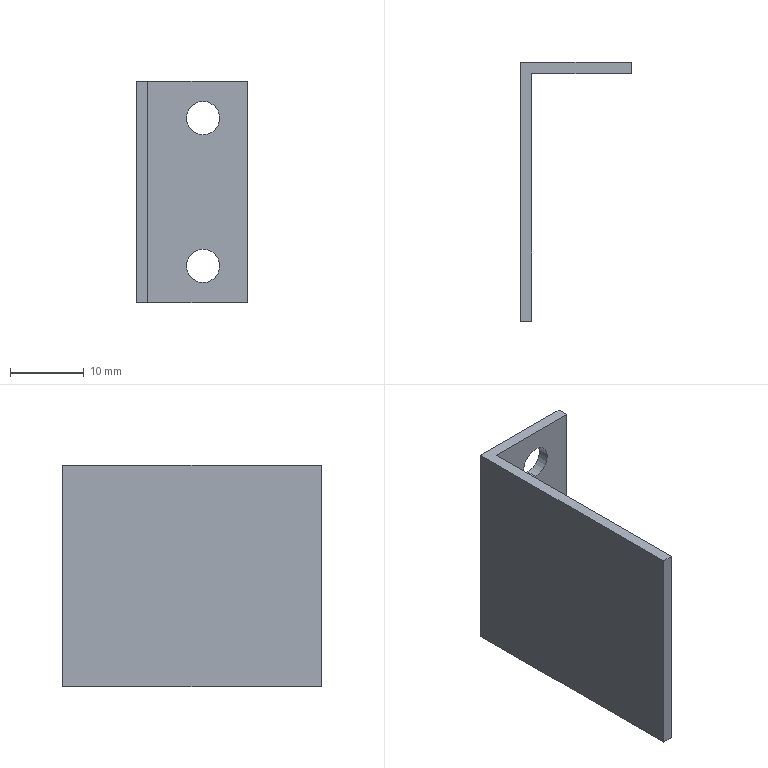Part | STEP file | 0245_210_Dog | 1 solid | 12 faces | box 15 x 35 x 30 mm | volume 2135 mm3 | plane 8 | cylinder 4 | commonest cylinder face diameters 4.5 x4
STEP:
#1=CARTESIAN_POINT('',(0.,0.,0.));
#2=DIRECTION('',(0.,0.,1.));
#3=DIRECTION('',(1.,0.,0.));
#4=AXIS2_PLACEMENT_3D('',#1,#2,#3);
#5=CARTESIAN_POINT('',(9.,-1.5,12.25));
#6=VERTEX_POINT('',#5);
#7=CARTESIAN_POINT('',(9.,0.,12.25));
#8=VERTEX_POINT('',#7);
#9=CARTESIAN_POINT('',(9.,0.,12.25));
#10=DIRECTION('',(0.,1.,0.));
#11=VECTOR('',#10,1.);
#12=LINE('',#9,#11);
#13=CARTESIAN_POINT('',(9.,0.,10.));
#14=DIRECTION('',(0.,1.,0.));
#15=DIRECTION('',(0.,0.,1.));
#16=AXIS2_PLACEMENT_3D('',#13,#14,#15);
#17=CYLINDRICAL_SURFACE('',#16,2.25);
#18=CARTESIAN_POINT('',(6.283,0.));
#19=DIRECTION('',(0.,1.));
#20=VECTOR('',#19,1.);
#21=LINE('',#18,#20);
#22=(GEOMETRIC_REPRESENTATION_CONTEXT(2)PARAMETRIC_REPRESENTATION_CONTEXT()REPRESENTATION_CONTEXT('',''));
#23=DEFINITIONAL_REPRESENTATION('',(#21),#22);
#24=PCURVE('',#17,#23);
#25=CARTESIAN_POINT('',(9.,0.,10.));
#26=DIRECTION('',(0.,1.,0.));
#27=DIRECTION('',(0.,0.,1.));
#28=AXIS2_PLACEMENT_3D('',#25,#26,#27);
#29=CYLINDRICAL_SURFACE('',#28,2.25);
#30=CARTESIAN_POINT('',(0.,0.));
#31=DIRECTION('',(0.,1.));
#32=VECTOR('',#31,1.);
#33=LINE('',#30,#32);
#34=(GEOMETRIC_REPRESENTATION_CONTEXT(2)PARAMETRIC_REPRESENTATION_CONTEXT()REPRESENTATION_CONTEXT('',''));
#35=DEFINITIONAL_REPRESENTATION('',(#33),#34);
#36=PCURVE('',#29,#35);
#37=SURFACE_CURVE('',#12,(#24,#36),.PCURVE_S1.);
#38=EDGE_CURVE('',#6,#8,#37,.T.);
#39=ORIENTED_EDGE('',*,*,#38,.T.);
#40=CARTESIAN_POINT('',(9.,0.,7.75));
#41=VERTEX_POINT('',#40);
#42=CARTESIAN_POINT('',(9.,0.,10.));
#43=DIRECTION('',(0.,1.,0.));
#44=DIRECTION('',(0.,0.,1.));
#45=AXIS2_PLACEMENT_3D('',#42,#43,#44);
#46=CIRCLE('',#45,2.25);
#47=CARTESIAN_POINT('',(0.,0.));
#48=DIRECTION('',(1.,0.));
#49=VECTOR('',#48,1.);
#50=LINE('',#47,#49);
#51=(GEOMETRIC_REPRESENTATION_CONTEXT(2)PARAMETRIC_REPRESENTATION_CONTEXT()REPRESENTATION_CONTEXT('',''));
#52=DEFINITIONAL_REPRESENTATION('',(#50),#51);
#53=PCURVE('',#17,#52);
#54=CARTESIAN_POINT('',(15.,0.,15.));
#55=DIRECTION('',(0.,-1.,0.));
#56=DIRECTION('',(1.,0.,0.));
#57=AXIS2_PLACEMENT_3D('',#54,#55,#56);
#58=PLANE('',#57);
#59=CARTESIAN_POINT('',(-6.,-2.75));
#60=CARTESIAN_POINT('',(-2.103,-2.75));
#61=CARTESIAN_POINT('',(-4.051,-6.125));
#62=CARTESIAN_POINT('',(-6.,-9.5));
#63=CARTESIAN_POINT('',(-7.949,-6.125));
#64=CARTESIAN_POINT('',(-9.897,-2.75));
#65=CARTESIAN_POINT('',(-6.,-2.75));
#66=(BOUNDED_CURVE()B_SPLINE_CURVE(2,(#59,#60,#61,#62,#63,#64,#65),.UNSPECIFIED.,.T.,.F.)B_SPLINE_CURVE_WITH_KNOTS((1,2,2,2,2,1),(-2.094,0.,2.094,4.189,6.283,8.378),.UNSPECIFIED.)CURVE()GEOMETRIC_REPRESENTATION_ITEM()RATIONAL_B_SPLINE_CURVE((1.,0.5,1.,0.5,1.,0.5,1.))REPRESENTATION_ITEM(''));
#67=(GEOMETRIC_REPRESENTATION_CONTEXT(2)PARAMETRIC_REPRESENTATION_CONTEXT()REPRESENTATION_CONTEXT('',''));
#68=DEFINITIONAL_REPRESENTATION('',(#66),#67);
#69=PCURVE('',#58,#68);
#70=SURFACE_CURVE('',#46,(#53,#69),.PCURVE_S1.);
#71=EDGE_CURVE('',#41,#8,#70,.T.);
#72=ORIENTED_EDGE('',*,*,#71,.F.);
#73=CARTESIAN_POINT('',(9.,-1.5,7.75));
#74=VERTEX_POINT('',#73);
#75=CARTESIAN_POINT('',(9.,0.,7.75));
#76=DIRECTION('',(0.,1.,0.));
#77=VECTOR('',#76,1.);
#78=LINE('',#75,#77);
#79=CARTESIAN_POINT('',(3.142,0.));
#80=DIRECTION('',(0.,1.));
#81=VECTOR('',#80,1.);
#82=LINE('',#79,#81);
#83=(GEOMETRIC_REPRESENTATION_CONTEXT(2)PARAMETRIC_REPRESENTATION_CONTEXT()REPRESENTATION_CONTEXT('',''));
#84=DEFINITIONAL_REPRESENTATION('',(#82),#83);
#85=PCURVE('',#17,#84);
#86=CARTESIAN_POINT('',(3.142,0.));
#87=DIRECTION('',(0.,1.));
#88=VECTOR('',#87,1.);
#89=LINE('',#86,#88);
#90=(GEOMETRIC_REPRESENTATION_CONTEXT(2)PARAMETRIC_REPRESENTATION_CONTEXT()REPRESENTATION_CONTEXT('',''));
#91=DEFINITIONAL_REPRESENTATION('',(#89),#90);
#92=PCURVE('',#29,#91);
#93=SURFACE_CURVE('',#78,(#85,#92),.PCURVE_S1.);
#94=EDGE_CURVE('',#74,#41,#93,.T.);
#95=ORIENTED_EDGE('',*,*,#94,.F.);
#96=CARTESIAN_POINT('',(9.,-1.5,10.));
#97=DIRECTION('',(0.,1.,0.));
#98=DIRECTION('',(-1.,0.,0.));
#99=AXIS2_PLACEMENT_3D('',#96,#97,#98);
#100=CIRCLE('',#99,2.25);
#101=CARTESIAN_POINT('',(-1.571,-1.5));
#102=DIRECTION('',(1.,0.));
#103=VECTOR('',#102,1.);
#104=LINE('',#101,#103);
#105=(GEOMETRIC_REPRESENTATION_CONTEXT(2)PARAMETRIC_REPRESENTATION_CONTEXT()REPRESENTATION_CONTEXT('',''));
#106=DEFINITIONAL_REPRESENTATION('',(#104),#105);
#107=PCURVE('',#17,#106);
#108=CARTESIAN_POINT('',(1.5,-1.5,15.));
#109=DIRECTION('',(0.,1.,0.));
#110=DIRECTION('',(-1.,0.,0.));
#111=AXIS2_PLACEMENT_3D('',#108,#109,#110);
#112=PLANE('',#111);
#113=CARTESIAN_POINT('',(-7.5,-5.));
#114=DIRECTION('',(1.,0.));
#115=AXIS2_PLACEMENT_2D('',#113,#114);
#116=CIRCLE('',#115,2.25);
#117=(GEOMETRIC_REPRESENTATION_CONTEXT(2)PARAMETRIC_REPRESENTATION_CONTEXT()REPRESENTATION_CONTEXT('',''));
#118=DEFINITIONAL_REPRESENTATION('',(#116),#117);
#119=PCURVE('',#112,#118);
#120=SURFACE_CURVE('',#100,(#107,#119),.PCURVE_S1.);
#121=EDGE_CURVE('',#74,#6,#120,.T.);
#122=ORIENTED_EDGE('',*,*,#121,.T.);
#123=EDGE_LOOP('',(#39,#72,#95,#122));
#124=FACE_BOUND('',#123,.F.);
#125=ADVANCED_FACE('',(#124),#17,.F.);
#126=CARTESIAN_POINT('',(9.,-1.5,-7.75));
#127=VERTEX_POINT('',#126);
#128=CARTESIAN_POINT('',(9.,0.,-7.75));
#129=VERTEX_POINT('',#128);
#130=CARTESIAN_POINT('',(9.,0.,-7.75));
#131=DIRECTION('',(0.,1.,0.));
#132=VECTOR('',#131,1.);
#133=LINE('',#130,#132);
#134=CARTESIAN_POINT('',(9.,0.,-10.));
#135=DIRECTION('',(0.,1.,0.));
#136=DIRECTION('',(0.,0.,1.));
#137=AXIS2_PLACEMENT_3D('',#134,#135,#136);
#138=CYLINDRICAL_SURFACE('',#137,2.25);
#139=CARTESIAN_POINT('',(6.283,0.));
#140=DIRECTION('',(0.,1.));
#141=VECTOR('',#140,1.);
#142=LINE('',#139,#141);
#143=(GEOMETRIC_REPRESENTATION_CONTEXT(2)PARAMETRIC_REPRESENTATION_CONTEXT()REPRESENTATION_CONTEXT('',''));
#144=DEFINITIONAL_REPRESENTATION('',(#142),#143);
#145=PCURVE('',#138,#144);
#146=CARTESIAN_POINT('',(9.,0.,-10.));
#147=DIRECTION('',(0.,1.,0.));
#148=DIRECTION('',(0.,0.,1.));
#149=AXIS2_PLACEMENT_3D('',#146,#147,#148);
#150=CYLINDRICAL_SURFACE('',#149,2.25);
#151=CARTESIAN_POINT('',(0.,0.));
#152=DIRECTION('',(0.,1.));
#153=VECTOR('',#152,1.);
#154=LINE('',#151,#153);
#155=(GEOMETRIC_REPRESENTATION_CONTEXT(2)PARAMETRIC_REPRESENTATION_CONTEXT()REPRESENTATION_CONTEXT('',''));
#156=DEFINITIONAL_REPRESENTATION('',(#154),#155);
#157=PCURVE('',#150,#156);
#158=SURFACE_CURVE('',#133,(#145,#157),.PCURVE_S1.);
#159=EDGE_CURVE('',#127,#129,#158,.T.);
#160=ORIENTED_EDGE('',*,*,#159,.T.);
#161=CARTESIAN_POINT('',(9.,0.,-12.25));
#162=VERTEX_POINT('',#161);
#163=CARTESIAN_POINT('',(9.,0.,-10.));
#164=DIRECTION('',(0.,1.,0.));
#165=DIRECTION('',(0.,0.,1.));
#166=AXIS2_PLACEMENT_3D('',#163,#164,#165);
#167=CIRCLE('',#166,2.25);
#168=CARTESIAN_POINT('',(0.,0.));
#169=DIRECTION('',(1.,0.));
#170=VECTOR('',#169,1.);
#171=LINE('',#168,#170);
#172=(GEOMETRIC_REPRESENTATION_CONTEXT(2)PARAMETRIC_REPRESENTATION_CONTEXT()REPRESENTATION_CONTEXT('',''));
#173=DEFINITIONAL_REPRESENTATION('',(#171),#172);
#174=PCURVE('',#138,#173);
#175=CARTESIAN_POINT('',(-6.,-22.75));
#176=CARTESIAN_POINT('',(-2.103,-22.75));
#177=CARTESIAN_POINT('',(-4.051,-26.125));
#178=CARTESIAN_POINT('',(-6.,-29.5));
#179=CARTESIAN_POINT('',(-7.949,-26.125));
#180=CARTESIAN_POINT('',(-9.897,-22.75));
#181=CARTESIAN_POINT('',(-6.,-22.75));
#182=(BOUNDED_CURVE()B_SPLINE_CURVE(2,(#175,#176,#177,#178,#179,#180,#181),.UNSPECIFIED.,.T.,.F.)B_SPLINE_CURVE_WITH_KNOTS((1,2,2,2,2,1),(-2.094,0.,2.094,4.189,6.283,8.378),.UNSPECIFIED.)CURVE()GEOMETRIC_REPRESENTATION_ITEM()RATIONAL_B_SPLINE_CURVE((1.,0.5,1.,0.5,1.,0.5,1.))REPRESENTATION_ITEM(''));
#183=(GEOMETRIC_REPRESENTATION_CONTEXT(2)PARAMETRIC_REPRESENTATION_CONTEXT()REPRESENTATION_CONTEXT('',''));
#184=DEFINITIONAL_REPRESENTATION('',(#182),#183);
#185=PCURVE('',#58,#184);
#186=SURFACE_CURVE('',#167,(#174,#185),.PCURVE_S1.);
#187=EDGE_CURVE('',#162,#129,#186,.T.);
#188=ORIENTED_EDGE('',*,*,#187,.F.);
#189=CARTESIAN_POINT('',(9.,-1.5,-12.25));
#190=VERTEX_POINT('',#189);
#191=CARTESIAN_POINT('',(9.,0.,-12.25));
#192=DIRECTION('',(0.,1.,0.));
#193=VECTOR('',#192,1.);
#194=LINE('',#191,#193);
#195=CARTESIAN_POINT('',(3.142,0.));
#196=DIRECTION('',(0.,1.));
#197=VECTOR('',#196,1.);
#198=LINE('',#195,#197);
#199=(GEOMETRIC_REPRESENTATION_CONTEXT(2)PARAMETRIC_REPRESENTATION_CONTEXT()REPRESENTATION_CONTEXT('',''));
#200=DEFINITIONAL_REPRESENTATION('',(#198),#199);
#201=PCURVE('',#138,#200);
#202=CARTESIAN_POINT('',(3.142,0.));
#203=DIRECTION('',(0.,1.));
#204=VECTOR('',#203,1.);
#205=LINE('',#202,#204);
#206=(GEOMETRIC_REPRESENTATION_CONTEXT(2)PARAMETRIC_REPRESENTATION_CONTEXT()REPRESENTATION_CONTEXT('',''));
#207=DEFINITIONAL_REPRESENTATION('',(#205),#206);
#208=PCURVE('',#150,#207);
#209=SURFACE_CURVE('',#194,(#201,#208),.PCURVE_S1.);
#210=EDGE_CURVE('',#190,#162,#209,.T.);
#211=ORIENTED_EDGE('',*,*,#210,.F.);
#212=CARTESIAN_POINT('',(9.,-1.5,-10.));
#213=DIRECTION('',(0.,1.,0.));
#214=DIRECTION('',(-1.,0.,0.));
#215=AXIS2_PLACEMENT_3D('',#212,#213,#214);
#216=CIRCLE('',#215,2.25);
#217=CARTESIAN_POINT('',(-1.571,-1.5));
#218=DIRECTION('',(1.,0.));
#219=VECTOR('',#218,1.);
#220=LINE('',#217,#219);
#221=(GEOMETRIC_REPRESENTATION_CONTEXT(2)PARAMETRIC_REPRESENTATION_CONTEXT()REPRESENTATION_CONTEXT('',''));
#222=DEFINITIONAL_REPRESENTATION('',(#220),#221);
#223=PCURVE('',#138,#222);
#224=CARTESIAN_POINT('',(-7.5,-25.));
#225=DIRECTION('',(1.,0.));
#226=AXIS2_PLACEMENT_2D('',#224,#225);
#227=CIRCLE('',#226,2.25);
#228=(GEOMETRIC_REPRESENTATION_CONTEXT(2)PARAMETRIC_REPRESENTATION_CONTEXT()REPRESENTATION_CONTEXT('',''));
#229=DEFINITIONAL_REPRESENTATION('',(#227),#228);
#230=PCURVE('',#112,#229);
#231=SURFACE_CURVE('',#216,(#223,#230),.PCURVE_S1.);
#232=EDGE_CURVE('',#190,#127,#231,.T.);
#233=ORIENTED_EDGE('',*,*,#232,.T.);
#234=EDGE_LOOP('',(#160,#188,#211,#233));
#235=FACE_BOUND('',#234,.F.);
#236=ADVANCED_FACE('',(#235),#138,.F.);
#237=CARTESIAN_POINT('',(9.,0.,10.));
#238=DIRECTION('',(0.,1.,0.));
#239=DIRECTION('',(0.,0.,1.));
#240=AXIS2_PLACEMENT_3D('',#237,#238,#239);
#241=CIRCLE('',#240,2.25);
#242=CARTESIAN_POINT('',(-6.,-2.75));
#243=CARTESIAN_POINT('',(-2.103,-2.75));
#244=CARTESIAN_POINT('',(-4.051,-6.125));
#245=CARTESIAN_POINT('',(-6.,-9.5));
#246=CARTESIAN_POINT('',(-7.949,-6.125));
#247=CARTESIAN_POINT('',(-9.897,-2.75));
#248=CARTESIAN_POINT('',(-6.,-2.75));
#249=(BOUNDED_CURVE()B_SPLINE_CURVE(2,(#242,#243,#244,#245,#246,#247,#248),.UNSPECIFIED.,.T.,.F.)B_SPLINE_CURVE_WITH_KNOTS((1,2,2,2,2,1),(-2.094,0.,2.094,4.189,6.283,8.378),.UNSPECIFIED.)CURVE()GEOMETRIC_REPRESENTATION_ITEM()RATIONAL_B_SPLINE_CURVE((1.,0.5,1.,0.5,1.,0.5,1.))REPRESENTATION_ITEM(''));
#250=(GEOMETRIC_REPRESENTATION_CONTEXT(2)PARAMETRIC_REPRESENTATION_CONTEXT()REPRESENTATION_CONTEXT('',''));
#251=DEFINITIONAL_REPRESENTATION('',(#249),#250);
#252=PCURVE('',#58,#251);
#253=CARTESIAN_POINT('',(0.,0.));
#254=DIRECTION('',(1.,0.));
#255=VECTOR('',#254,1.);
#256=LINE('',#253,#255);
#257=(GEOMETRIC_REPRESENTATION_CONTEXT(2)PARAMETRIC_REPRESENTATION_CONTEXT()REPRESENTATION_CONTEXT('',''));
#258=DEFINITIONAL_REPRESENTATION('',(#256),#257);
#259=PCURVE('',#29,#258);
#260=SURFACE_CURVE('',#241,(#252,#259),.PCURVE_S1.);
#261=EDGE_CURVE('',#8,#41,#260,.T.);
#262=ORIENTED_EDGE('',*,*,#261,.F.);
#263=ORIENTED_EDGE('',*,*,#71,.F.);
#264=EDGE_LOOP('',(#262,#263));
#265=FACE_BOUND('',#264,.T.);
#266=CARTESIAN_POINT('',(9.,0.,-10.));
#267=DIRECTION('',(0.,1.,0.));
#268=DIRECTION('',(0.,0.,1.));
#269=AXIS2_PLACEMENT_3D('',#266,#267,#268);
#270=CIRCLE('',#269,2.25);
#271=CARTESIAN_POINT('',(-6.,-22.75));
#272=CARTESIAN_POINT('',(-2.103,-22.75));
#273=CARTESIAN_POINT('',(-4.051,-26.125));
#274=CARTESIAN_POINT('',(-6.,-29.5));
#275=CARTESIAN_POINT('',(-7.949,-26.125));
#276=CARTESIAN_POINT('',(-9.897,-22.75));
#277=CARTESIAN_POINT('',(-6.,-22.75));
#278=(BOUNDED_CURVE()B_SPLINE_CURVE(2,(#271,#272,#273,#274,#275,#276,#277),.UNSPECIFIED.,.T.,.F.)B_SPLINE_CURVE_WITH_KNOTS((1,2,2,2,2,1),(-2.094,0.,2.094,4.189,6.283,8.378),.UNSPECIFIED.)CURVE()GEOMETRIC_REPRESENTATION_ITEM()RATIONAL_B_SPLINE_CURVE((1.,0.5,1.,0.5,1.,0.5,1.))REPRESENTATION_ITEM(''));
#279=(GEOMETRIC_REPRESENTATION_CONTEXT(2)PARAMETRIC_REPRESENTATION_CONTEXT()REPRESENTATION_CONTEXT('',''));
#280=DEFINITIONAL_REPRESENTATION('',(#278),#279);
#281=PCURVE('',#58,#280);
#282=CARTESIAN_POINT('',(0.,0.));
#283=DIRECTION('',(1.,0.));
#284=VECTOR('',#283,1.);
#285=LINE('',#282,#284);
#286=(GEOMETRIC_REPRESENTATION_CONTEXT(2)PARAMETRIC_REPRESENTATION_CONTEXT()REPRESENTATION_CONTEXT('',''));
#287=DEFINITIONAL_REPRESENTATION('',(#285),#286);
#288=PCURVE('',#150,#287);
#289=SURFACE_CURVE('',#270,(#281,#288),.PCURVE_S1.);
#290=EDGE_CURVE('',#129,#162,#289,.T.);
#291=ORIENTED_EDGE('',*,*,#290,.F.);
#292=ORIENTED_EDGE('',*,*,#187,.F.);
#293=EDGE_LOOP('',(#291,#292));
#294=FACE_BOUND('',#293,.T.);
#295=CARTESIAN_POINT('',(15.,0.,-15.));
#296=VERTEX_POINT('',#295);
#297=CARTESIAN_POINT('',(0.,0.,-15.));
#298=VERTEX_POINT('',#297);
#299=CARTESIAN_POINT('',(15.,0.,-15.));
#300=DIRECTION('',(-1.,0.,0.));
#301=VECTOR('',#300,1.);
#302=LINE('',#299,#301);
#303=CARTESIAN_POINT('',(0.,-30.));
#304=DIRECTION('',(-1.,0.));
#305=VECTOR('',#304,1.);
#306=LINE('',#303,#305);
#307=(GEOMETRIC_REPRESENTATION_CONTEXT(2)PARAMETRIC_REPRESENTATION_CONTEXT()REPRESENTATION_CONTEXT('',''));
#308=DEFINITIONAL_REPRESENTATION('',(#306),#307);
#309=PCURVE('',#58,#308);
#310=CARTESIAN_POINT('',(0.,0.,-15.));
#311=DIRECTION('',(0.,0.,1.));
#312=DIRECTION('',(1.,0.,0.));
#313=AXIS2_PLACEMENT_3D('',#310,#311,#312);
#314=PLANE('',#313);
#315=CARTESIAN_POINT('',(15.,0.));
#316=DIRECTION('',(-1.,0.));
#317=VECTOR('',#316,1.);
#318=LINE('',#315,#317);
#319=(GEOMETRIC_REPRESENTATION_CONTEXT(2)PARAMETRIC_REPRESENTATION_CONTEXT()REPRESENTATION_CONTEXT('',''));
#320=DEFINITIONAL_REPRESENTATION('',(#318),#319);
#321=PCURVE('',#314,#320);
#322=SURFACE_CURVE('',#302,(#309,#321),.PCURVE_S1.);
#323=EDGE_CURVE('',#296,#298,#322,.T.);
#324=ORIENTED_EDGE('',*,*,#323,.T.);
#325=CARTESIAN_POINT('',(0.,0.,15.));
#326=VERTEX_POINT('',#325);
#327=CARTESIAN_POINT('',(0.,0.,15.));
#328=DIRECTION('',(0.,0.,-1.));
#329=VECTOR('',#328,1.);
#330=LINE('',#327,#329);
#331=CARTESIAN_POINT('',(-15.,0.));
#332=DIRECTION('',(0.,-1.));
#333=VECTOR('',#332,1.);
#334=LINE('',#331,#333);
#335=(GEOMETRIC_REPRESENTATION_CONTEXT(2)PARAMETRIC_REPRESENTATION_CONTEXT()REPRESENTATION_CONTEXT('',''));
#336=DEFINITIONAL_REPRESENTATION('',(#334),#335);
#337=PCURVE('',#58,#336);
#338=CARTESIAN_POINT('',(0.,0.,15.));
#339=DIRECTION('',(1.,0.,0.));
#340=DIRECTION('',(0.,1.,0.));
#341=AXIS2_PLACEMENT_3D('',#338,#339,#340);
#342=PLANE('',#341);
#343=CARTESIAN_POINT('',(0.,0.));
#344=DIRECTION('',(0.,-1.));
#345=VECTOR('',#344,1.);
#346=LINE('',#343,#345);
#347=(GEOMETRIC_REPRESENTATION_CONTEXT(2)PARAMETRIC_REPRESENTATION_CONTEXT()REPRESENTATION_CONTEXT('',''));
#348=DEFINITIONAL_REPRESENTATION('',(#346),#347);
#349=PCURVE('',#342,#348);
#350=SURFACE_CURVE('',#330,(#337,#349),.PCURVE_S1.);
#351=EDGE_CURVE('',#326,#298,#350,.T.);
#352=ORIENTED_EDGE('',*,*,#351,.F.);
#353=CARTESIAN_POINT('',(15.,0.,15.));
#354=VERTEX_POINT('',#353);
#355=CARTESIAN_POINT('',(15.,0.,15.));
#356=DIRECTION('',(-1.,0.,0.));
#357=VECTOR('',#356,1.);
#358=LINE('',#355,#357);
#359=CARTESIAN_POINT('',(0.,0.));
#360=DIRECTION('',(-1.,0.));
#361=VECTOR('',#360,1.);
#362=LINE('',#359,#361);
#363=(GEOMETRIC_REPRESENTATION_CONTEXT(2)PARAMETRIC_REPRESENTATION_CONTEXT()REPRESENTATION_CONTEXT('',''));
#364=DEFINITIONAL_REPRESENTATION('',(#362),#363);
#365=PCURVE('',#58,#364);
#366=CARTESIAN_POINT('',(0.,0.,15.));
#367=DIRECTION('',(0.,0.,1.));
#368=DIRECTION('',(1.,0.,0.));
#369=AXIS2_PLACEMENT_3D('',#366,#367,#368);
#370=PLANE('',#369);
#371=CARTESIAN_POINT('',(15.,0.));
#372=DIRECTION('',(-1.,0.));
#373=VECTOR('',#372,1.);
#374=LINE('',#371,#373);
#375=(GEOMETRIC_REPRESENTATION_CONTEXT(2)PARAMETRIC_REPRESENTATION_CONTEXT()REPRESENTATION_CONTEXT('',''));
#376=DEFINITIONAL_REPRESENTATION('',(#374),#375);
#377=PCURVE('',#370,#376);
#378=SURFACE_CURVE('',#358,(#365,#377),.PCURVE_S1.);
#379=EDGE_CURVE('',#354,#326,#378,.T.);
#380=ORIENTED_EDGE('',*,*,#379,.F.);
#381=CARTESIAN_POINT('',(15.,0.,15.));
#382=DIRECTION('',(0.,0.,-1.));
#383=VECTOR('',#382,1.);
#384=LINE('',#381,#383);
#385=CARTESIAN_POINT('',(0.,0.));
#386=DIRECTION('',(0.,-1.));
#387=VECTOR('',#386,1.);
#388=LINE('',#385,#387);
#389=(GEOMETRIC_REPRESENTATION_CONTEXT(2)PARAMETRIC_REPRESENTATION_CONTEXT()REPRESENTATION_CONTEXT('',''));
#390=DEFINITIONAL_REPRESENTATION('',(#388),#389);
#391=PCURVE('',#58,#390);
#392=CARTESIAN_POINT('',(15.,-1.5,15.));
#393=DIRECTION('',(-1.,0.,0.));
#394=DIRECTION('',(0.,0.,1.));
#395=AXIS2_PLACEMENT_3D('',#392,#393,#394);
#396=PLANE('',#395);
#397=CARTESIAN_POINT('',(0.,1.5));
#398=DIRECTION('',(-1.,0.));
#399=VECTOR('',#398,1.);
#400=LINE('',#397,#399);
#401=(GEOMETRIC_REPRESENTATION_CONTEXT(2)PARAMETRIC_REPRESENTATION_CONTEXT()REPRESENTATION_CONTEXT('',''));
#402=DEFINITIONAL_REPRESENTATION('',(#400),#401);
#403=PCURVE('',#396,#402);
#404=SURFACE_CURVE('',#384,(#391,#403),.PCURVE_S1.);
#405=EDGE_CURVE('',#354,#296,#404,.T.);
#406=ORIENTED_EDGE('',*,*,#405,.T.);
#407=EDGE_LOOP('',(#324,#352,#380,#406));
#408=FACE_BOUND('',#407,.T.);
#409=ADVANCED_FACE('',(#265,#294,#408),#58,.F.);
#410=CARTESIAN_POINT('',(0.,-35.,-15.));
#411=VERTEX_POINT('',#410);
#412=CARTESIAN_POINT('',(0.,0.,-15.));
#413=DIRECTION('',(0.,-1.,0.));
#414=VECTOR('',#413,1.);
#415=LINE('',#412,#414);
#416=CARTESIAN_POINT('',(0.,-30.));
#417=DIRECTION('',(-1.,0.));
#418=VECTOR('',#417,1.);
#419=LINE('',#416,#418);
#420=(GEOMETRIC_REPRESENTATION_CONTEXT(2)PARAMETRIC_REPRESENTATION_CONTEXT()REPRESENTATION_CONTEXT('',''));
#421=DEFINITIONAL_REPRESENTATION('',(#419),#420);
#422=PCURVE('',#342,#421);
#423=CARTESIAN_POINT('',(0.,0.));
#424=DIRECTION('',(0.,-1.));
#425=VECTOR('',#424,1.);
#426=LINE('',#423,#425);
#427=(GEOMETRIC_REPRESENTATION_CONTEXT(2)PARAMETRIC_REPRESENTATION_CONTEXT()REPRESENTATION_CONTEXT('',''));
#428=DEFINITIONAL_REPRESENTATION('',(#426),#427);
#429=PCURVE('',#314,#428);
#430=SURFACE_CURVE('',#415,(#422,#429),.PCURVE_S1.);
#431=EDGE_CURVE('',#298,#411,#430,.T.);
#432=ORIENTED_EDGE('',*,*,#431,.T.);
#433=CARTESIAN_POINT('',(0.,-35.,15.));
#434=VERTEX_POINT('',#433);
#435=CARTESIAN_POINT('',(0.,-35.,15.));
#436=DIRECTION('',(0.,0.,-1.));
#437=VECTOR('',#436,1.);
#438=LINE('',#435,#437);
#439=CARTESIAN_POINT('',(-35.,0.));
#440=DIRECTION('',(0.,-1.));
#441=VECTOR('',#440,1.);
#442=LINE('',#439,#441);
#443=(GEOMETRIC_REPRESENTATION_CONTEXT(2)PARAMETRIC_REPRESENTATION_CONTEXT()REPRESENTATION_CONTEXT('',''));
#444=DEFINITIONAL_REPRESENTATION('',(#442),#443);
#445=PCURVE('',#342,#444);
#446=CARTESIAN_POINT('',(0.,-35.,15.));
#447=DIRECTION('',(0.,1.,0.));
#448=DIRECTION('',(0.,0.,1.));
#449=AXIS2_PLACEMENT_3D('',#446,#447,#448);
#450=PLANE('',#449);
#451=CARTESIAN_POINT('',(0.,0.));
#452=DIRECTION('',(-1.,0.));
#453=VECTOR('',#452,1.);
#454=LINE('',#451,#453);
#455=(GEOMETRIC_REPRESENTATION_CONTEXT(2)PARAMETRIC_REPRESENTATION_CONTEXT()REPRESENTATION_CONTEXT('',''));
#456=DEFINITIONAL_REPRESENTATION('',(#454),#455);
#457=PCURVE('',#450,#456);
#458=SURFACE_CURVE('',#438,(#445,#457),.PCURVE_S1.);
#459=EDGE_CURVE('',#434,#411,#458,.T.);
#460=ORIENTED_EDGE('',*,*,#459,.F.);
#461=CARTESIAN_POINT('',(0.,0.,15.));
#462=DIRECTION('',(0.,-1.,0.));
#463=VECTOR('',#462,1.);
#464=LINE('',#461,#463);
#465=CARTESIAN_POINT('',(0.,0.));
#466=DIRECTION('',(-1.,0.));
#467=VECTOR('',#466,1.);
#468=LINE('',#465,#467);
#469=(GEOMETRIC_REPRESENTATION_CONTEXT(2)PARAMETRIC_REPRESENTATION_CONTEXT()REPRESENTATION_CONTEXT('',''));
#470=DEFINITIONAL_REPRESENTATION('',(#468),#469);
#471=PCURVE('',#342,#470);
#472=CARTESIAN_POINT('',(0.,0.));
#473=DIRECTION('',(0.,-1.));
#474=VECTOR('',#473,1.);
#475=LINE('',#472,#474);
#476=(GEOMETRIC_REPRESENTATION_CONTEXT(2)PARAMETRIC_REPRESENTATION_CONTEXT()REPRESENTATION_CONTEXT('',''));
#477=DEFINITIONAL_REPRESENTATION('',(#475),#476);
#478=PCURVE('',#370,#477);
#479=SURFACE_CURVE('',#464,(#471,#478),.PCURVE_S1.);
#480=EDGE_CURVE('',#326,#434,#479,.T.);
#481=ORIENTED_EDGE('',*,*,#480,.F.);
#482=ORIENTED_EDGE('',*,*,#351,.T.);
#483=EDGE_LOOP('',(#432,#460,#481,#482));
#484=FACE_BOUND('',#483,.T.);
#485=ADVANCED_FACE('',(#484),#342,.F.);
#486=CARTESIAN_POINT('',(1.5,-35.,-15.));
#487=VERTEX_POINT('',#486);
#488=CARTESIAN_POINT('',(0.,-35.,-15.));
#489=DIRECTION('',(1.,0.,0.));
#490=VECTOR('',#489,1.);
#491=LINE('',#488,#490);
#492=CARTESIAN_POINT('',(-30.,0.));
#493=DIRECTION('',(0.,1.));
#494=VECTOR('',#493,1.);
#495=LINE('',#492,#494);
#496=(GEOMETRIC_REPRESENTATION_CONTEXT(2)PARAMETRIC_REPRESENTATION_CONTEXT()REPRESENTATION_CONTEXT('',''));
#497=DEFINITIONAL_REPRESENTATION('',(#495),#496);
#498=PCURVE('',#450,#497);
#499=CARTESIAN_POINT('',(0.,-35.));
#500=DIRECTION('',(1.,0.));
#501=VECTOR('',#500,1.);
#502=LINE('',#499,#501);
#503=(GEOMETRIC_REPRESENTATION_CONTEXT(2)PARAMETRIC_REPRESENTATION_CONTEXT()REPRESENTATION_CONTEXT('',''));
#504=DEFINITIONAL_REPRESENTATION('',(#502),#503);
#505=PCURVE('',#314,#504);
#506=SURFACE_CURVE('',#491,(#498,#505),.PCURVE_S1.);
#507=EDGE_CURVE('',#411,#487,#506,.T.);
#508=ORIENTED_EDGE('',*,*,#507,.T.);
#509=CARTESIAN_POINT('',(1.5,-35.,15.));
#510=VERTEX_POINT('',#509);
#511=CARTESIAN_POINT('',(1.5,-35.,15.));
#512=DIRECTION('',(0.,0.,-1.));
#513=VECTOR('',#512,1.);
#514=LINE('',#511,#513);
#515=CARTESIAN_POINT('',(0.,1.5));
#516=DIRECTION('',(-1.,0.));
#517=VECTOR('',#516,1.);
#518=LINE('',#515,#517);
#519=(GEOMETRIC_REPRESENTATION_CONTEXT(2)PARAMETRIC_REPRESENTATION_CONTEXT()REPRESENTATION_CONTEXT('',''));
#520=DEFINITIONAL_REPRESENTATION('',(#518),#519);
#521=PCURVE('',#450,#520);
#522=CARTESIAN_POINT('',(1.5,-35.,15.));
#523=DIRECTION('',(-1.,0.,0.));
#524=DIRECTION('',(0.,-1.,0.));
#525=AXIS2_PLACEMENT_3D('',#522,#523,#524);
#526=PLANE('',#525);
#527=CARTESIAN_POINT('',(0.,0.));
#528=DIRECTION('',(0.,-1.));
#529=VECTOR('',#528,1.);
#530=LINE('',#527,#529);
#531=(GEOMETRIC_REPRESENTATION_CONTEXT(2)PARAMETRIC_REPRESENTATION_CONTEXT()REPRESENTATION_CONTEXT('',''));
#532=DEFINITIONAL_REPRESENTATION('',(#530),#531);
#533=PCURVE('',#526,#532);
#534=SURFACE_CURVE('',#514,(#521,#533),.PCURVE_S1.);
#535=EDGE_CURVE('',#510,#487,#534,.T.);
#536=ORIENTED_EDGE('',*,*,#535,.F.);
#537=CARTESIAN_POINT('',(0.,-35.,15.));
#538=DIRECTION('',(1.,0.,0.));
#539=VECTOR('',#538,1.);
#540=LINE('',#537,#539);
#541=CARTESIAN_POINT('',(0.,0.));
#542=DIRECTION('',(0.,1.));
#543=VECTOR('',#542,1.);
#544=LINE('',#541,#543);
#545=(GEOMETRIC_REPRESENTATION_CONTEXT(2)PARAMETRIC_REPRESENTATION_CONTEXT()REPRESENTATION_CONTEXT('',''));
#546=DEFINITIONAL_REPRESENTATION('',(#544),#545);
#547=PCURVE('',#450,#546);
#548=CARTESIAN_POINT('',(0.,-35.));
#549=DIRECTION('',(1.,0.));
#550=VECTOR('',#549,1.);
#551=LINE('',#548,#550);
#552=(GEOMETRIC_REPRESENTATION_CONTEXT(2)PARAMETRIC_REPRESENTATION_CONTEXT()REPRESENTATION_CONTEXT('',''));
#553=DEFINITIONAL_REPRESENTATION('',(#551),#552);
#554=PCURVE('',#370,#553);
#555=SURFACE_CURVE('',#540,(#547,#554),.PCURVE_S1.);
#556=EDGE_CURVE('',#434,#510,#555,.T.);
#557=ORIENTED_EDGE('',*,*,#556,.F.);
#558=ORIENTED_EDGE('',*,*,#459,.T.);
#559=EDGE_LOOP('',(#508,#536,#557,#558));
#560=FACE_BOUND('',#559,.T.);
#561=ADVANCED_FACE('',(#560),#450,.F.);
#562=CARTESIAN_POINT('',(1.5,-1.5,-15.));
#563=VERTEX_POINT('',#562);
#564=CARTESIAN_POINT('',(1.5,-35.,-15.));
#565=DIRECTION('',(0.,1.,0.));
#566=VECTOR('',#565,1.);
#567=LINE('',#564,#566);
#568=CARTESIAN_POINT('',(0.,-30.));
#569=DIRECTION('',(-1.,0.));
#570=VECTOR('',#569,1.);
#571=LINE('',#568,#570);
#572=(GEOMETRIC_REPRESENTATION_CONTEXT(2)PARAMETRIC_REPRESENTATION_CONTEXT()REPRESENTATION_CONTEXT('',''));
#573=DEFINITIONAL_REPRESENTATION('',(#571),#572);
#574=PCURVE('',#526,#573);
#575=CARTESIAN_POINT('',(1.5,-35.));
#576=DIRECTION('',(0.,1.));
#577=VECTOR('',#576,1.);
#578=LINE('',#575,#577);
#579=(GEOMETRIC_REPRESENTATION_CONTEXT(2)PARAMETRIC_REPRESENTATION_CONTEXT()REPRESENTATION_CONTEXT('',''));
#580=DEFINITIONAL_REPRESENTATION('',(#578),#579);
#581=PCURVE('',#314,#580);
#582=SURFACE_CURVE('',#567,(#574,#581),.PCURVE_S1.);
#583=EDGE_CURVE('',#487,#563,#582,.T.);
#584=ORIENTED_EDGE('',*,*,#583,.T.);
#585=CARTESIAN_POINT('',(1.5,-1.5,15.));
#586=VERTEX_POINT('',#585);
#587=CARTESIAN_POINT('',(1.5,-1.5,15.));
#588=DIRECTION('',(0.,0.,-1.));
#589=VECTOR('',#588,1.);
#590=LINE('',#587,#589);
#591=CARTESIAN_POINT('',(-33.5,0.));
#592=DIRECTION('',(0.,-1.));
#593=VECTOR('',#592,1.);
#594=LINE('',#591,#593);
#595=(GEOMETRIC_REPRESENTATION_CONTEXT(2)PARAMETRIC_REPRESENTATION_CONTEXT()REPRESENTATION_CONTEXT('',''));
#596=DEFINITIONAL_REPRESENTATION('',(#594),#595);
#597=PCURVE('',#526,#596);
#598=CARTESIAN_POINT('',(0.,0.));
#599=DIRECTION('',(0.,-1.));
#600=VECTOR('',#599,1.);
#601=LINE('',#598,#600);
#602=(GEOMETRIC_REPRESENTATION_CONTEXT(2)PARAMETRIC_REPRESENTATION_CONTEXT()REPRESENTATION_CONTEXT('',''));
#603=DEFINITIONAL_REPRESENTATION('',(#601),#602);
#604=PCURVE('',#112,#603);
#605=SURFACE_CURVE('',#590,(#597,#604),.PCURVE_S1.);
#606=EDGE_CURVE('',#586,#563,#605,.T.);
#607=ORIENTED_EDGE('',*,*,#606,.F.);
#608=CARTESIAN_POINT('',(1.5,-35.,15.));
#609=DIRECTION('',(0.,1.,0.));
#610=VECTOR('',#609,1.);
#611=LINE('',#608,#610);
#612=CARTESIAN_POINT('',(0.,0.));
#613=DIRECTION('',(-1.,0.));
#614=VECTOR('',#613,1.);
#615=LINE('',#612,#614);
#616=(GEOMETRIC_REPRESENTATION_CONTEXT(2)PARAMETRIC_REPRESENTATION_CONTEXT()REPRESENTATION_CONTEXT('',''));
#617=DEFINITIONAL_REPRESENTATION('',(#615),#616);
#618=PCURVE('',#526,#617);
#619=CARTESIAN_POINT('',(1.5,-35.));
#620=DIRECTION('',(0.,1.));
#621=VECTOR('',#620,1.);
#622=LINE('',#619,#621);
#623=(GEOMETRIC_REPRESENTATION_CONTEXT(2)PARAMETRIC_REPRESENTATION_CONTEXT()REPRESENTATION_CONTEXT('',''));
#624=DEFINITIONAL_REPRESENTATION('',(#622),#623);
#625=PCURVE('',#370,#624);
#626=SURFACE_CURVE('',#611,(#618,#625),.PCURVE_S1.);
#627=EDGE_CURVE('',#510,#586,#626,.T.);
#628=ORIENTED_EDGE('',*,*,#627,.F.);
#629=ORIENTED_EDGE('',*,*,#535,.T.);
#630=EDGE_LOOP('',(#584,#607,#628,#629));
#631=FACE_BOUND('',#630,.T.);
#632=ADVANCED_FACE('',(#631),#526,.F.);
#633=CARTESIAN_POINT('',(9.,-1.5,10.));
#634=DIRECTION('',(0.,1.,0.));
#635=DIRECTION('',(-1.,0.,0.));
#636=AXIS2_PLACEMENT_3D('',#633,#634,#635);
#637=CIRCLE('',#636,2.25);
#638=CARTESIAN_POINT('',(-7.5,-5.));
#639=DIRECTION('',(1.,0.));
#640=AXIS2_PLACEMENT_2D('',#638,#639);
#641=CIRCLE('',#640,2.25);
#642=(GEOMETRIC_REPRESENTATION_CONTEXT(2)PARAMETRIC_REPRESENTATION_CONTEXT()REPRESENTATION_CONTEXT('',''));
#643=DEFINITIONAL_REPRESENTATION('',(#641),#642);
#644=PCURVE('',#112,#643);
#645=CARTESIAN_POINT('',(-1.571,-1.5));
#646=DIRECTION('',(1.,0.));
#647=VECTOR('',#646,1.);
#648=LINE('',#645,#647);
#649=(GEOMETRIC_REPRESENTATION_CONTEXT(2)PARAMETRIC_REPRESENTATION_CONTEXT()REPRESENTATION_CONTEXT('',''));
#650=DEFINITIONAL_REPRESENTATION('',(#648),#649);
#651=PCURVE('',#29,#650);
#652=SURFACE_CURVE('',#637,(#644,#651),.PCURVE_S1.);
#653=EDGE_CURVE('',#6,#74,#652,.T.);
#654=ORIENTED_EDGE('',*,*,#653,.T.);
#655=ORIENTED_EDGE('',*,*,#121,.T.);
#656=EDGE_LOOP('',(#654,#655));
#657=FACE_BOUND('',#656,.T.);
#658=CARTESIAN_POINT('',(9.,-1.5,-10.));
#659=DIRECTION('',(0.,1.,0.));
#660=DIRECTION('',(-1.,0.,0.));
#661=AXIS2_PLACEMENT_3D('',#658,#659,#660);
#662=CIRCLE('',#661,2.25);
#663=CARTESIAN_POINT('',(-7.5,-25.));
#664=DIRECTION('',(1.,0.));
#665=AXIS2_PLACEMENT_2D('',#663,#664);
#666=CIRCLE('',#665,2.25);
#667=(GEOMETRIC_REPRESENTATION_CONTEXT(2)PARAMETRIC_REPRESENTATION_CONTEXT()REPRESENTATION_CONTEXT('',''));
#668=DEFINITIONAL_REPRESENTATION('',(#666),#667);
#669=PCURVE('',#112,#668);
#670=CARTESIAN_POINT('',(-1.571,-1.5));
#671=DIRECTION('',(1.,0.));
#672=VECTOR('',#671,1.);
#673=LINE('',#670,#672);
#674=(GEOMETRIC_REPRESENTATION_CONTEXT(2)PARAMETRIC_REPRESENTATION_CONTEXT()REPRESENTATION_CONTEXT('',''));
#675=DEFINITIONAL_REPRESENTATION('',(#673),#674);
#676=PCURVE('',#150,#675);
#677=SURFACE_CURVE('',#662,(#669,#676),.PCURVE_S1.);
#678=EDGE_CURVE('',#127,#190,#677,.T.);
#679=ORIENTED_EDGE('',*,*,#678,.T.);
#680=ORIENTED_EDGE('',*,*,#232,.T.);
#681=EDGE_LOOP('',(#679,#680));
#682=FACE_BOUND('',#681,.T.);
#683=CARTESIAN_POINT('',(15.,-1.5,-15.));
#684=VERTEX_POINT('',#683);
#685=CARTESIAN_POINT('',(1.5,-1.5,-15.));
#686=DIRECTION('',(1.,0.,0.));
#687=VECTOR('',#686,1.);
#688=LINE('',#685,#687);
#689=CARTESIAN_POINT('',(0.,-30.));
#690=DIRECTION('',(-1.,0.));
#691=VECTOR('',#690,1.);
#692=LINE('',#689,#691);
#693=(GEOMETRIC_REPRESENTATION_CONTEXT(2)PARAMETRIC_REPRESENTATION_CONTEXT()REPRESENTATION_CONTEXT('',''));
#694=DEFINITIONAL_REPRESENTATION('',(#692),#693);
#695=PCURVE('',#112,#694);
#696=CARTESIAN_POINT('',(1.5,-1.5));
#697=DIRECTION('',(1.,0.));
#698=VECTOR('',#697,1.);
#699=LINE('',#696,#698);
#700=(GEOMETRIC_REPRESENTATION_CONTEXT(2)PARAMETRIC_REPRESENTATION_CONTEXT()REPRESENTATION_CONTEXT('',''));
#701=DEFINITIONAL_REPRESENTATION('',(#699),#700);
#702=PCURVE('',#314,#701);
#703=SURFACE_CURVE('',#688,(#695,#702),.PCURVE_S1.);
#704=EDGE_CURVE('',#563,#684,#703,.T.);
#705=ORIENTED_EDGE('',*,*,#704,.T.);
#706=CARTESIAN_POINT('',(15.,-1.5,15.));
#707=VERTEX_POINT('',#706);
#708=CARTESIAN_POINT('',(15.,-1.5,15.));
#709=DIRECTION('',(0.,0.,-1.));
#710=VECTOR('',#709,1.);
#711=LINE('',#708,#710);
#712=CARTESIAN_POINT('',(-13.5,0.));
#713=DIRECTION('',(0.,-1.));
#714=VECTOR('',#713,1.);
#715=LINE('',#712,#714);
#716=(GEOMETRIC_REPRESENTATION_CONTEXT(2)PARAMETRIC_REPRESENTATION_CONTEXT()REPRESENTATION_CONTEXT('',''));
#717=DEFINITIONAL_REPRESENTATION('',(#715),#716);
#718=PCURVE('',#112,#717);
#719=CARTESIAN_POINT('',(0.,0.));
#720=DIRECTION('',(-1.,0.));
#721=VECTOR('',#720,1.);
#722=LINE('',#719,#721);
#723=(GEOMETRIC_REPRESENTATION_CONTEXT(2)PARAMETRIC_REPRESENTATION_CONTEXT()REPRESENTATION_CONTEXT('',''));
#724=DEFINITIONAL_REPRESENTATION('',(#722),#723);
#725=PCURVE('',#396,#724);
#726=SURFACE_CURVE('',#711,(#718,#725),.PCURVE_S1.);
#727=EDGE_CURVE('',#707,#684,#726,.T.);
#728=ORIENTED_EDGE('',*,*,#727,.F.);
#729=CARTESIAN_POINT('',(1.5,-1.5,15.));
#730=DIRECTION('',(1.,0.,0.));
#731=VECTOR('',#730,1.);
#732=LINE('',#729,#731);
#733=CARTESIAN_POINT('',(0.,0.));
#734=DIRECTION('',(-1.,0.));
#735=VECTOR('',#734,1.);
#736=LINE('',#733,#735);
#737=(GEOMETRIC_REPRESENTATION_CONTEXT(2)PARAMETRIC_REPRESENTATION_CONTEXT()REPRESENTATION_CONTEXT('',''));
#738=DEFINITIONAL_REPRESENTATION('',(#736),#737);
#739=PCURVE('',#112,#738);
#740=CARTESIAN_POINT('',(1.5,-1.5));
#741=DIRECTION('',(1.,0.));
#742=VECTOR('',#741,1.);
#743=LINE('',#740,#742);
#744=(GEOMETRIC_REPRESENTATION_CONTEXT(2)PARAMETRIC_REPRESENTATION_CONTEXT()REPRESENTATION_CONTEXT('',''));
#745=DEFINITIONAL_REPRESENTATION('',(#743),#744);
#746=PCURVE('',#370,#745);
#747=SURFACE_CURVE('',#732,(#739,#746),.PCURVE_S1.);
#748=EDGE_CURVE('',#586,#707,#747,.T.);
#749=ORIENTED_EDGE('',*,*,#748,.F.);
#750=ORIENTED_EDGE('',*,*,#606,.T.);
#751=EDGE_LOOP('',(#705,#728,#749,#750));
#752=FACE_BOUND('',#751,.T.);
#753=ADVANCED_FACE('',(#657,#682,#752),#112,.F.);
#754=CARTESIAN_POINT('',(15.,-1.5,-15.));
#755=DIRECTION('',(0.,1.,0.));
#756=VECTOR('',#755,1.);
#757=LINE('',#754,#756);
#758=CARTESIAN_POINT('',(-30.,0.));
#759=DIRECTION('',(0.,1.));
#760=VECTOR('',#759,1.);
#761=LINE('',#758,#760);
#762=(GEOMETRIC_REPRESENTATION_CONTEXT(2)PARAMETRIC_REPRESENTATION_CONTEXT()REPRESENTATION_CONTEXT('',''));
#763=DEFINITIONAL_REPRESENTATION('',(#761),#762);
#764=PCURVE('',#396,#763);
#765=CARTESIAN_POINT('',(15.,-1.5));
#766=DIRECTION('',(0.,1.));
#767=VECTOR('',#766,1.);
#768=LINE('',#765,#767);
#769=(GEOMETRIC_REPRESENTATION_CONTEXT(2)PARAMETRIC_REPRESENTATION_CONTEXT()REPRESENTATION_CONTEXT('',''));
#770=DEFINITIONAL_REPRESENTATION('',(#768),#769);
#771=PCURVE('',#314,#770);
#772=SURFACE_CURVE('',#757,(#764,#771),.PCURVE_S1.);
#773=EDGE_CURVE('',#684,#296,#772,.T.);
#774=ORIENTED_EDGE('',*,*,#773,.T.);
#775=ORIENTED_EDGE('',*,*,#405,.F.);
#776=CARTESIAN_POINT('',(15.,-1.5,15.));
#777=DIRECTION('',(0.,1.,0.));
#778=VECTOR('',#777,1.);
#779=LINE('',#776,#778);
#780=CARTESIAN_POINT('',(0.,0.));
#781=DIRECTION('',(0.,1.));
#782=VECTOR('',#781,1.);
#783=LINE('',#780,#782);
#784=(GEOMETRIC_REPRESENTATION_CONTEXT(2)PARAMETRIC_REPRESENTATION_CONTEXT()REPRESENTATION_CONTEXT('',''));
#785=DEFINITIONAL_REPRESENTATION('',(#783),#784);
#786=PCURVE('',#396,#785);
#787=CARTESIAN_POINT('',(15.,-1.5));
#788=DIRECTION('',(0.,1.));
#789=VECTOR('',#788,1.);
#790=LINE('',#787,#789);
#791=(GEOMETRIC_REPRESENTATION_CONTEXT(2)PARAMETRIC_REPRESENTATION_CONTEXT()REPRESENTATION_CONTEXT('',''));
#792=DEFINITIONAL_REPRESENTATION('',(#790),#791);
#793=PCURVE('',#370,#792);
#794=SURFACE_CURVE('',#779,(#786,#793),.PCURVE_S1.);
#795=EDGE_CURVE('',#707,#354,#794,.T.);
#796=ORIENTED_EDGE('',*,*,#795,.F.);
#797=ORIENTED_EDGE('',*,*,#727,.T.);
#798=EDGE_LOOP('',(#774,#775,#796,#797));
#799=FACE_BOUND('',#798,.T.);
#800=ADVANCED_FACE('',(#799),#396,.F.);
#801=ORIENTED_EDGE('',*,*,#379,.T.);
#802=ORIENTED_EDGE('',*,*,#480,.T.);
#803=ORIENTED_EDGE('',*,*,#556,.T.);
#804=ORIENTED_EDGE('',*,*,#627,.T.);
#805=ORIENTED_EDGE('',*,*,#748,.T.);
#806=ORIENTED_EDGE('',*,*,#795,.T.);
#807=EDGE_LOOP('',(#801,#802,#803,#804,#805,#806));
#808=FACE_BOUND('',#807,.T.);
#809=ADVANCED_FACE('',(#808),#370,.T.);
#810=ORIENTED_EDGE('',*,*,#323,.F.);
#811=ORIENTED_EDGE('',*,*,#773,.F.);
#812=ORIENTED_EDGE('',*,*,#704,.F.);
#813=ORIENTED_EDGE('',*,*,#583,.F.);
#814=ORIENTED_EDGE('',*,*,#507,.F.);
#815=ORIENTED_EDGE('',*,*,#431,.F.);
#816=EDGE_LOOP('',(#810,#811,#812,#813,#814,#815));
#817=FACE_BOUND('',#816,.T.);
#818=ADVANCED_FACE('',(#817),#314,.F.);
#819=ORIENTED_EDGE('',*,*,#290,.F.);
#820=ORIENTED_EDGE('',*,*,#159,.F.);
#821=ORIENTED_EDGE('',*,*,#678,.T.);
#822=ORIENTED_EDGE('',*,*,#210,.T.);
#823=EDGE_LOOP('',(#819,#820,#821,#822));
#824=FACE_BOUND('',#823,.F.);
#825=ADVANCED_FACE('',(#824),#150,.F.);
#826=ORIENTED_EDGE('',*,*,#261,.F.);
#827=ORIENTED_EDGE('',*,*,#38,.F.);
#828=ORIENTED_EDGE('',*,*,#653,.T.);
#829=ORIENTED_EDGE('',*,*,#94,.T.);
#830=EDGE_LOOP('',(#826,#827,#828,#829));
#831=FACE_BOUND('',#830,.F.);
#832=ADVANCED_FACE('',(#831),#29,.F.);
#833=CLOSED_SHELL('',(#125,#236,#409,#485,#561,#632,#753,#800,#809,#818,#825,#832));
#834=MANIFOLD_SOLID_BREP('',#833);
#835=(LENGTH_UNIT()NAMED_UNIT(*)SI_UNIT(.MILLI.,.METRE.));
#836=UNCERTAINTY_MEASURE_WITH_UNIT(LENGTH_MEASURE(0.0000001),#835,'','');
#837=(NAMED_UNIT(*)PLANE_ANGLE_UNIT()SI_UNIT($,.RADIAN.));
#838=(NAMED_UNIT(*)SI_UNIT($,.STERADIAN.)SOLID_ANGLE_UNIT());
#839=(GEOMETRIC_REPRESENTATION_CONTEXT(3)GLOBAL_UNCERTAINTY_ASSIGNED_CONTEXT((#836))GLOBAL_UNIT_ASSIGNED_CONTEXT((#835,#837,#838))REPRESENTATION_CONTEXT('',''));
#840=ADVANCED_BREP_SHAPE_REPRESENTATION('',(#4,#834),#839);